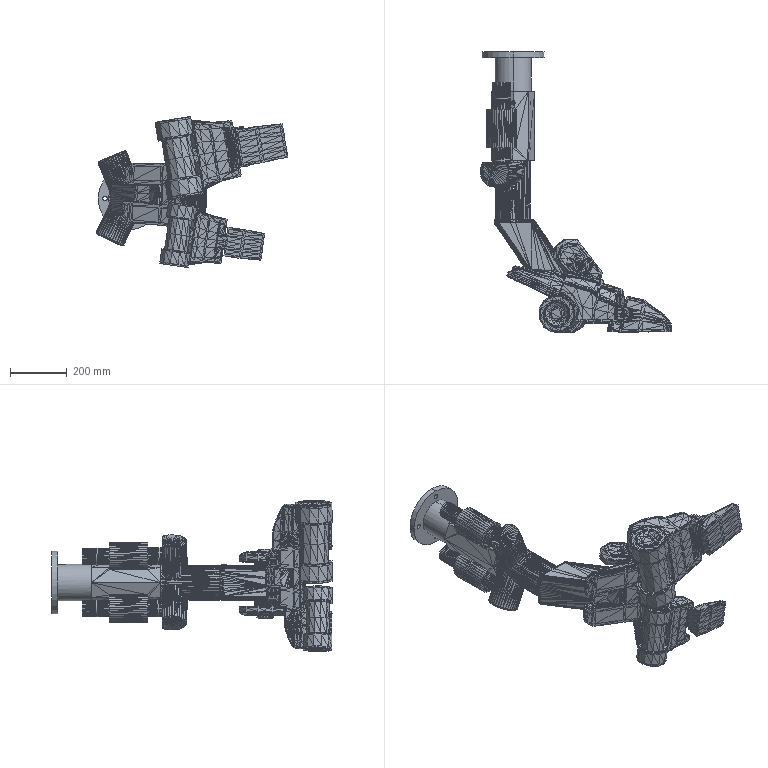Part | SolidWorks | features MirrorStock 1 | 1 solid | 14276 faces | volume 34150920 mm3 | plane 14241 | cylinder 35 | commonest cylinder face diameters 8 x16 16 x8 12 x4 14 x3 128 x2 220 x2